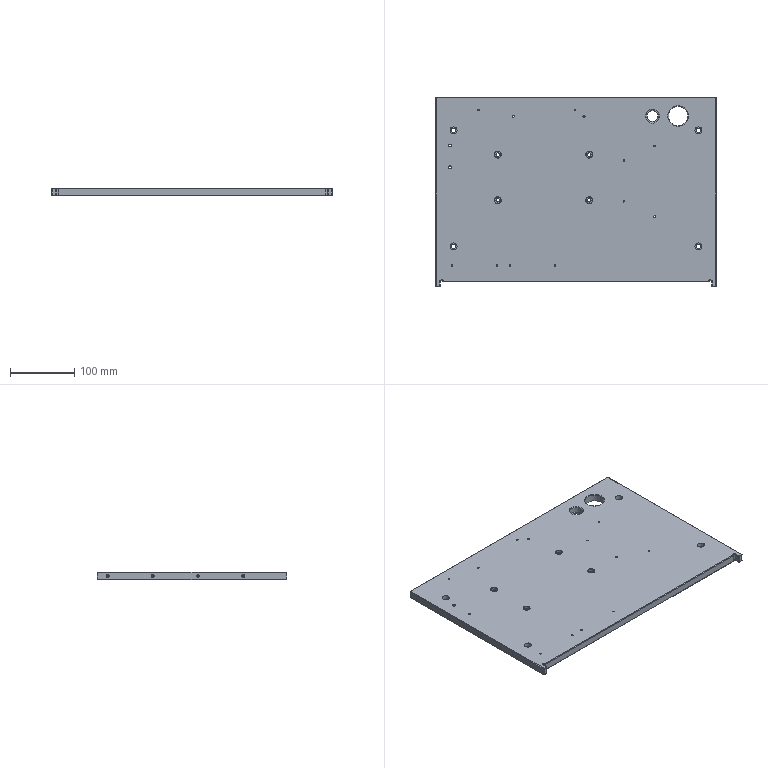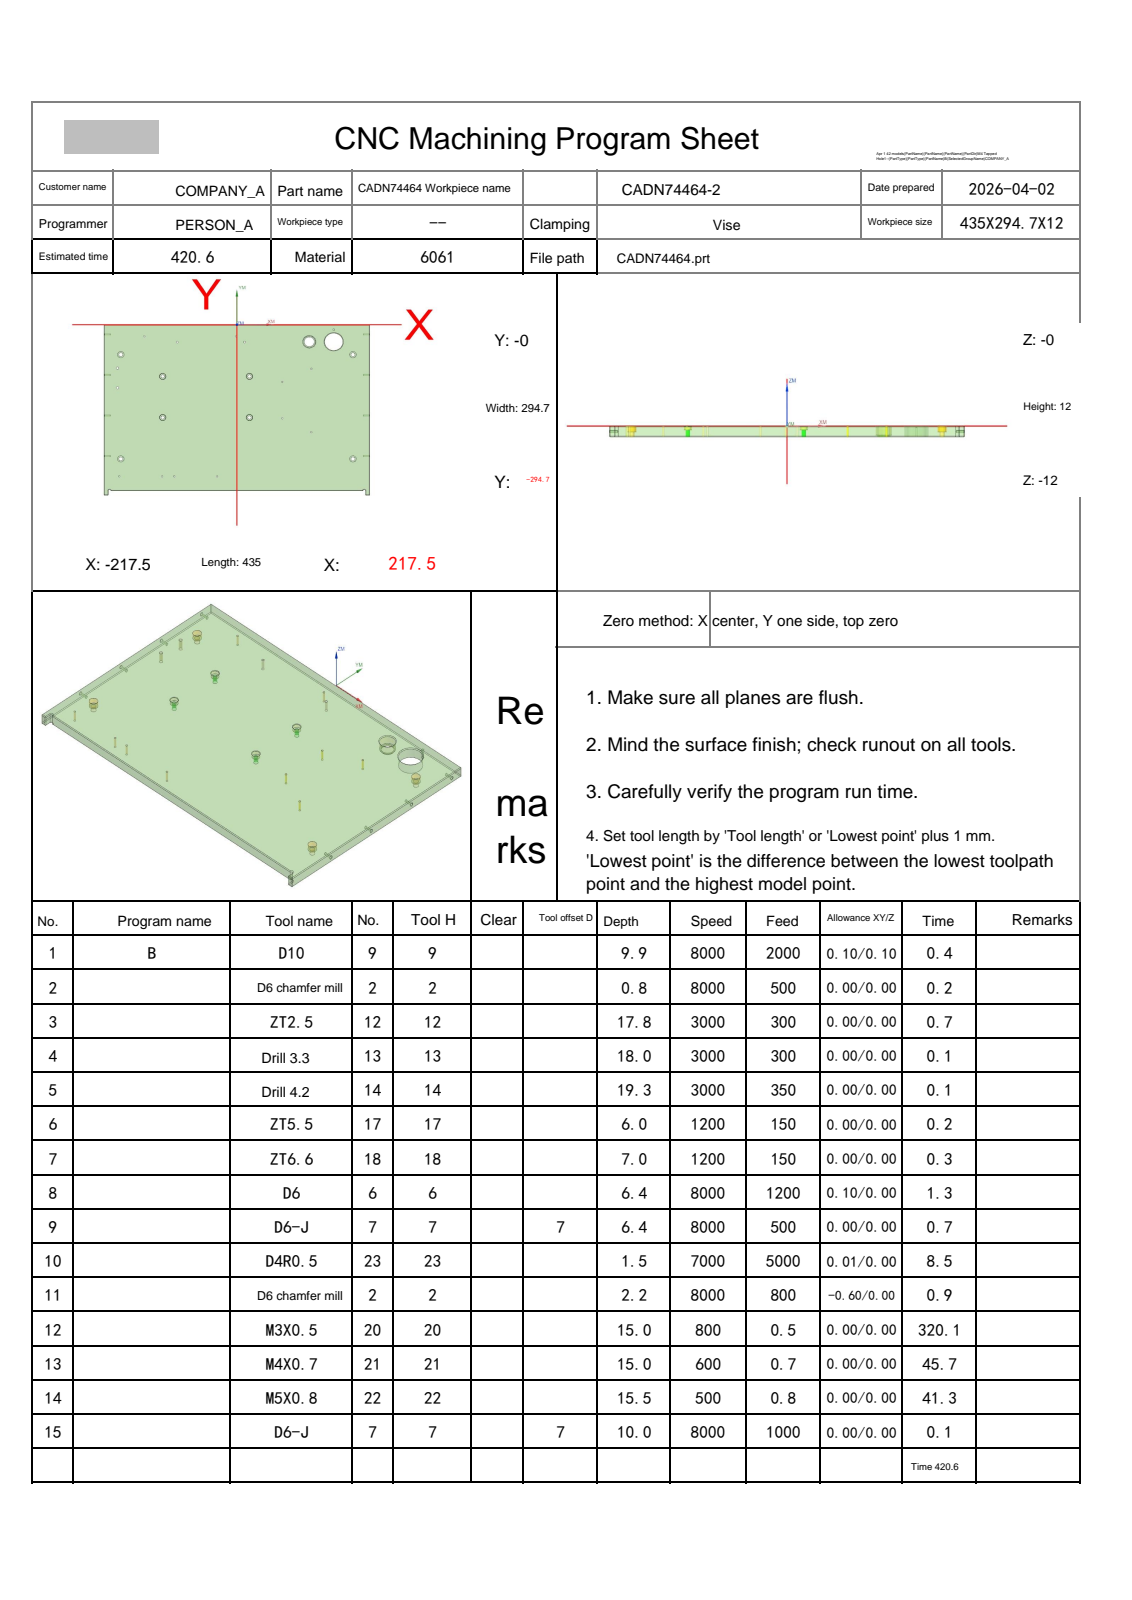NC program | NX | posted by the shop | part box 435 x 294.7 x 12 mm
Lines 634 to 1915 of 33933:
N10 T23 M06
(D4R0.5  D=4. R=0.5 H=23 ce=0.01 di=0.00)
G00 G90 G54 X119.057 Y-38.818 M03 S7000
G43 H23 Z20.
M08
Z1.5
G01 X119.198 Y-38.814 Z1.493 F5000.
X120.02 Y-38.715 Z1.449
X120.831 Y-38.544 Z1.406
X121.624 Y-38.302 Z1.362
X122.392 Y-37.991 Z1.319
X123.129 Y-37.612 Z1.276
X123.83 Y-37.17 Z1.232
X124.488 Y-36.668 Z1.189
X125.1 Y-36.109 Z1.145
X125.66 Y-35.498 Z1.102
X126.163 Y-34.839 Z1.058
X126.496 Y-34.327 Z1.026
X126.905 Y-33.574 Z.981
X127.243 Y-32.786 Z.937
X127.507 Y-31.971 Z.892
X127.696 Y-31.136 Z.847
X127.807 Y-30.286 Z.802
X127.84 Y-29.43 Z.757
X127.794 Y-28.574 Z.712
X127.67 Y-27.727 Z.667
X127.469 Y-26.894 Z.622
X127.192 Y-26.083 Z.577
X126.843 Y-25.301 Z.532
X126.423 Y-24.554 Z.488
X125.936 Y-23.849 Z.443
X125.387 Y-23.191 Z.398
X124.78 Y-22.586 Z.353
X124.12 Y-22.04 Z.308
X123.413 Y-21.556 Z.263
X122.664 Y-21.14 Z.218
X121.881 Y-20.793 Z.173
X121.068 Y-20.52 Z.128
X120.476 Y-20.371 Z.096
X119.645 Y-20.23 Z.052
X118.806 Y-20.165 Z.008
X118.5 Z-.008
G03 X109.165 Y-29.5 I0.0 J-9.335
X118.5 Y-38.835 I9.335 J0.0
X127.835 Y-29.5 I0.0 J9.335
X118.5 Y-20.165 I-9.335 J0.0
G01 X118.269 Y-20.168
X118.038 Y-20.177
X117.802 Y-20.192
X117.567 Y-20.213
X117.27 Y-20.248
X116.974 Y-20.293
X116.675 Y-20.348
X116.378 Y-20.413
X116.083 Y-20.488 Z-.009
X115.791 Y-20.572
X115.502 Y-20.665
X115.216 Y-20.768
X114.934 Y-20.88
X114.655 Y-21.002
X114.518 Y-21.066
X114.381 Y-21.132
X114.245 Y-21.2
X114.111 Y-21.271
X113.978 Y-21.344
X113.846 Y-21.419
X113.715 Y-21.496
X113.585 Y-21.575
X113.457 Y-21.657
X113.33 Y-21.74
X113.205 Y-21.826
X113.081 Y-21.913
X112.958 Y-22.003
X112.836 Y-22.094
X112.717 Y-22.187
X112.599 Y-22.283
X112.482 Y-22.38
X112.367 Y-22.479
X112.254 Y-22.58 Z-.01
X112.142 Y-22.683
X112.032 Y-22.788
X111.924 Y-22.894
X111.817 Y-23.002
X111.713 Y-23.113
X111.61 Y-23.224
X111.509 Y-23.337
X111.41 Y-23.452
X111.312 Y-23.569
X111.217 Y-23.687
X111.123 Y-23.806
X111.032 Y-23.927
X110.942 Y-24.05
X110.855 Y-24.174
X110.769 Y-24.299
X110.686 Y-24.426
X110.604 Y-24.554
X110.448 Y-24.814
X110.3 Y-25.079
X110.161 Y-25.348
X110.031 Y-25.622
X109.909 Y-25.901
X109.797 Y-26.182
X109.694 Y-26.468 Z-.011
X109.601 Y-26.756
X109.517 Y-27.048
X109.442 Y-27.342
X109.377 Y-27.638
X109.322 Y-27.936
X109.276 Y-28.236
X109.24 Y-28.537
X109.215 Y-28.839
X109.198 Y-29.142
X109.192 Y-29.445
X109.196 Y-29.748
X109.21 Y-30.051
X109.233 Y-30.353
X109.266 Y-30.655
X109.309 Y-30.955 Z-.012
X109.362 Y-31.253
X109.424 Y-31.55
X109.497 Y-31.844
X109.578 Y-32.136
X109.669 Y-32.425
X109.769 Y-32.711
X109.879 Y-32.993
X109.998 Y-33.272
X110.126 Y-33.546
X110.263 Y-33.817
X110.408 Y-34.082
X110.562 Y-34.343
X110.577 Y-34.367
X110.592 Y-34.392
X110.74 Y-34.623
X110.895 Y-34.849
X111.073 Y-35.093
X111.26 Y-35.332 Z-.013
X111.454 Y-35.564
X111.655 Y-35.79
X111.864 Y-36.009
X112.079 Y-36.221
X112.302 Y-36.426
X112.531 Y-36.623
X112.648 Y-36.719
X112.766 Y-36.813
X112.886 Y-36.906
X113.007 Y-36.996
X113.13 Y-37.084
X113.254 Y-37.17
X113.38 Y-37.254
X113.507 Y-37.336
X113.635 Y-37.416
X113.765 Y-37.494
X113.896 Y-37.57
X114.028 Y-37.643
X114.161 Y-37.715
X114.295 Y-37.785
X114.431 Y-37.852
X114.568 Y-37.916
X114.705 Y-37.979
X114.844 Y-38.04 Z-.014
X114.983 Y-38.098
X115.124 Y-38.153
X115.265 Y-38.207
X115.407 Y-38.258
X115.55 Y-38.307
X115.694 Y-38.354
X115.839 Y-38.398
X115.984 Y-38.44
X116.13 Y-38.48
X116.276 Y-38.517
X116.423 Y-38.551
X116.571 Y-38.584
X116.719 Y-38.614
X116.868 Y-38.641
X117.017 Y-38.666
X117.166 Y-38.689
X117.316 Y-38.709
X117.466 Y-38.727
X117.616 Y-38.743
X117.767 Y-38.756
X117.917 Y-38.766
X118.068 Y-38.774
X118.37 Y-38.783
X118.672 Y-38.782
X118.974 Y-38.771
X119.276 Y-38.75 Z-.015
X119.576 Y-38.719
X119.876 Y-38.679
X120.173 Y-38.629
X120.47 Y-38.569
X120.763 Y-38.5
X121.055 Y-38.421
X121.344 Y-38.333
X121.63 Y-38.235
X121.912 Y-38.128
X122.191 Y-38.012
X122.466 Y-37.887
X122.736 Y-37.753
X123.002 Y-37.61
X123.264 Y-37.459
X123.52 Y-37.3
X123.771 Y-37.132 Z-.016
X124.016 Y-36.956
X124.256 Y-36.772
X124.489 Y-36.581
X124.716 Y-36.382
X124.936 Y-36.175
X125.15 Y-35.962
X125.356 Y-35.742
X125.555 Y-35.515
X125.747 Y-35.282
X125.931 Y-35.043
X126.089 Y-34.823
X126.242 Y-34.598
X126.258 Y-34.573
X126.275 Y-34.548
X126.43 Y-34.298
X126.578 Y-34.045
X126.718 Y-33.786 Z-.017
X126.849 Y-33.524
X126.972 Y-33.257
X127.086 Y-32.987
X127.192 Y-32.713
X127.289 Y-32.436
X127.377 Y-32.156
X127.457 Y-31.873
X127.527 Y-31.588
X127.588 Y-31.301
X127.64 Y-31.012
X127.683 Y-30.722
X127.716 Y-30.431
X127.741 Y-30.138
X127.756 Y-29.845
X127.762 Y-29.552
X127.759 Y-29.258 Z-.018
X127.746 Y-28.965
X127.724 Y-28.673
X127.693 Y-28.381
X127.652 Y-28.091
X127.602 Y-27.801
X127.544 Y-27.514
X127.476 Y-27.229
X127.399 Y-26.946
X127.313 Y-26.665
X127.219 Y-26.388
X127.115 Y-26.113
X127.003 Y-25.842
X126.883 Y-25.575
X126.754 Y-25.311
X126.617 Y-25.052
X126.472 Y-24.798 Z-.019
X126.318 Y-24.548
X126.157 Y-24.303
X125.988 Y-24.063
X125.812 Y-23.829
X125.628 Y-23.6
X125.438 Y-23.378
X125.24 Y-23.161
X125.036 Y-22.951
X124.825 Y-22.748
X124.607 Y-22.551
X124.384 Y-22.362
X124.155 Y-22.179
X123.92 Y-22.004
X123.679 Y-21.836
X123.434 Y-21.677
X123.183 Y-21.525 Z-.02
X122.928 Y-21.381
X122.669 Y-21.245
X122.405 Y-21.117
X122.137 Y-20.998
X121.866 Y-20.887
X121.591 Y-20.786
X121.314 Y-20.692
X121.033 Y-20.608
X120.75 Y-20.532
X120.553 Y-20.486
X120.355 Y-20.443
X120.275 Y-20.428
X120.195 Y-20.412
X119.915 Y-20.365
X119.634 Y-20.326
X119.351 Y-20.296
X119.068 Y-20.274
X118.784 Y-20.262 Z-.021
X118.5 Y-20.258
X118.269 Y-20.261
X118.038 Y-20.27
X117.802 Y-20.285
X117.567 Y-20.306
X117.272 Y-20.342
X116.978 Y-20.386
X116.682 Y-20.441
X116.387 Y-20.506
X116.095 Y-20.58
X115.805 Y-20.664
X115.518 Y-20.757 Z-.022
X115.234 Y-20.86
X114.954 Y-20.972
X114.678 Y-21.093
X114.541 Y-21.156
X114.406 Y-21.222
X114.271 Y-21.291
X114.138 Y-21.361
X114.006 Y-21.433
X113.875 Y-21.508
X113.745 Y-21.585
X113.617 Y-21.664
X113.489 Y-21.745
X113.364 Y-21.828
X113.239 Y-21.913
X113.116 Y-22.
X112.995 Y-22.089
X112.874 Y-22.18
X112.756 Y-22.273 Z-.023
X112.639 Y-22.368
X112.523 Y-22.465
X112.409 Y-22.564
X112.297 Y-22.664
X112.187 Y-22.767
X112.078 Y-22.871
X111.97 Y-22.977
X111.865 Y-23.085
X111.761 Y-23.194
X111.659 Y-23.305
X111.559 Y-23.418
X111.461 Y-23.532
X111.365 Y-23.648
X111.271 Y-23.765
X111.178 Y-23.884
X111.088 Y-24.005
X110.999 Y-24.127
X110.828 Y-24.375
X110.665 Y-24.628
X110.511 Y-24.887 Z-.024
X110.365 Y-25.15
X110.228 Y-25.418
X110.099 Y-25.691
X109.98 Y-25.967
X109.869 Y-26.248
X109.768 Y-26.531
X109.676 Y-26.818
X109.594 Y-27.108
X109.521 Y-27.4
X109.458 Y-27.694
X109.404 Y-27.991 Z-.025
X109.36 Y-28.288
X109.326 Y-28.588
X109.302 Y-28.888
X109.287 Y-29.188
X109.283 Y-29.489
X109.287 Y-29.79
X109.302 Y-30.091
X109.327 Y-30.391
X109.362 Y-30.69
X109.406 Y-30.987
X109.46 Y-31.283 Z-.026
X109.523 Y-31.578
X109.596 Y-31.869
X109.679 Y-32.159
X109.771 Y-32.445
X109.872 Y-32.728
X109.983 Y-33.008
X110.102 Y-33.284
X110.231 Y-33.556
X110.368 Y-33.824
X110.514 Y-34.087
X110.668 Y-34.345 Z-.027
X110.683 Y-34.368
X110.697 Y-34.392
X110.845 Y-34.618
X110.998 Y-34.84
X111.175 Y-35.08
X111.36 Y-35.314
X111.552 Y-35.541
X111.751 Y-35.762
X111.958 Y-35.977
X112.171 Y-36.185
X112.391 Y-36.385
X112.617 Y-36.579
X112.849 Y-36.765 Z-.028
X113.087 Y-36.944
X113.331 Y-37.115
X113.58 Y-37.277
X113.835 Y-37.432
X114.094 Y-37.578
X114.358 Y-37.716
X114.626 Y-37.845
X114.898 Y-37.966
X115.174 Y-38.077
X115.313 Y-38.13
X115.453 Y-38.18
X115.594 Y-38.228 Z-.029
X115.735 Y-38.273
X115.878 Y-38.317
X116.021 Y-38.358
X116.164 Y-38.397
X116.308 Y-38.433
X116.453 Y-38.467
X116.599 Y-38.499
X116.744 Y-38.528
X116.891 Y-38.555
X117.037 Y-38.58
X117.184 Y-38.602
X117.332 Y-38.622
X117.479 Y-38.639
X117.776 Y-38.667
X118.072 Y-38.685
X118.37 Y-38.694
X118.667 Y-38.693
X118.964 Y-38.682 Z-.03
X119.261 Y-38.662
X119.557 Y-38.632
X119.851 Y-38.593
X120.145 Y-38.544
X120.436 Y-38.486
X120.726 Y-38.418
X121.013 Y-38.341
X121.297 Y-38.254
X121.579 Y-38.159
X121.857 Y-38.055
X122.132 Y-37.941 Z-.031
X122.402 Y-37.819
X122.669 Y-37.688
X122.931 Y-37.548
X123.189 Y-37.401
X123.442 Y-37.244
X123.69 Y-37.08
X123.932 Y-36.908
X124.168 Y-36.728
X124.399 Y-36.541
X124.623 Y-36.346
X124.841 Y-36.144 Z-.032
X125.052 Y-35.935
X125.256 Y-35.72
X125.454 Y-35.498
X125.644 Y-35.269
X125.826 Y-35.035
X126.001 Y-34.795
X126.168 Y-34.55
X126.224 Y-34.463
X126.279 Y-34.377
X126.381 Y-34.209
X126.479 Y-34.04
X126.622 Y-33.778
X126.757 Y-33.512 Z-.033
X126.882 Y-33.241
X126.999 Y-32.966
X127.107 Y-32.688
X127.206 Y-32.406
X127.295 Y-32.121
X127.375 Y-31.834
X127.446 Y-31.544
X127.507 Y-31.252
X127.559 Y-30.958
X127.601 Y-30.663
X127.634 Y-30.366 Z-.034
X127.657 Y-30.069
X127.67 Y-29.771
X127.674 Y-29.472
X127.667 Y-29.174
X127.652 Y-28.876
X127.626 Y-28.579
X127.591 Y-28.283
X127.546 Y-27.988
X127.492 Y-27.695
X127.428 Y-27.404
X127.355 Y-27.115 Z-.035
X127.272 Y-26.828
X127.18 Y-26.544
X127.079 Y-26.264
X126.969 Y-25.987
X126.85 Y-25.713
X126.722 Y-25.444
X126.585 Y-25.179
X126.44 Y-24.919
X126.364 Y-24.79
X126.287 Y-24.663
X126.207 Y-24.537
X126.125 Y-24.413
X126.041 Y-24.29
X125.955 Y-24.168 Z-.036
X125.867 Y-24.048
X125.777 Y-23.929
X125.686 Y-23.811
X125.592 Y-23.695
X125.497 Y-23.581
X125.399 Y-23.468
X125.3 Y-23.357
X125.199 Y-23.247
X125.097 Y-23.139
X124.992 Y-23.033
X124.886 Y-22.928
X124.778 Y-22.825
X124.669 Y-22.724
X124.558 Y-22.625
X124.331 Y-22.432
X124.097 Y-22.247
X123.859 Y-22.069
X123.614 Y-21.899 Z-.037
X123.364 Y-21.737
X123.109 Y-21.583
X122.849 Y-21.438
X122.584 Y-21.301
X122.315 Y-21.173
X122.042 Y-21.054
X121.766 Y-20.943
X121.485 Y-20.842
X121.202 Y-20.75
X120.916 Y-20.667
X120.628 Y-20.594 Z-.038
X120.337 Y-20.53
X120.11 Y-20.487
X119.882 Y-20.449
X119.864 Y-20.447
X119.847 Y-20.444
X119.635 Y-20.415
X119.423 Y-20.391
X119.193 Y-20.371
X118.962 Y-20.357
X118.731 Y-20.349
X118.5 Y-20.346
X118.269 Y-20.349
X118.038 Y-20.358
X117.807 Y-20.374
X117.576 Y-20.394 Z-.039
X117.461 Y-20.407
X117.345 Y-20.421
X117.164 Y-20.446
X116.983 Y-20.475
X116.688 Y-20.53
X116.396 Y-20.595
X116.106 Y-20.669
X115.818 Y-20.752
X115.533 Y-20.845
X115.252 Y-20.948
X114.974 Y-21.059 Z-.04
X114.7 Y-21.179
X114.564 Y-21.243
X114.43 Y-21.309
X114.296 Y-21.377
X114.164 Y-21.447
X114.033 Y-21.519
X113.903 Y-21.593
X113.774 Y-21.67
X113.647 Y-21.749
X113.521 Y-21.829
X113.396 Y-21.912
X113.273 Y-21.997
X113.151 Y-22.084
X113.03 Y-22.172
X112.911 Y-22.263 Z-.041
X112.793 Y-22.356
X112.678 Y-22.45
X112.563 Y-22.547
X112.45 Y-22.645
X112.339 Y-22.745
X112.229 Y-22.847
X112.121 Y-22.951
X112.015 Y-23.056
X111.911 Y-23.163
X111.808 Y-23.272
X111.707 Y-23.383
X111.608 Y-23.495
X111.511 Y-23.609
X111.416 Y-23.724
X111.231 Y-23.959
X111.054 Y-24.2 Z-.042
X110.885 Y-24.447
X110.724 Y-24.699
X110.571 Y-24.957
X110.427 Y-25.219
X110.292 Y-25.486
X110.165 Y-25.757
X110.048 Y-26.032
X109.939 Y-26.31
X109.84 Y-26.592 Z-.043
X109.75 Y-26.877
X109.669 Y-27.165
X109.598 Y-27.456
X109.536 Y-27.748
X109.484 Y-28.043
X109.442 Y-28.339
X109.409 Y-28.636
X109.386 Y-28.934 Z-.044
X109.373 Y-29.233
X109.37 Y-29.531
X109.376 Y-29.83
X109.392 Y-30.129
X109.418 Y-30.426
X109.454 Y-30.723
X109.499 Y-31.019
X109.554 Y-31.312
X109.618 Y-31.604 Z-.045
X109.693 Y-31.893
X109.776 Y-32.18
X109.869 Y-32.464
X109.971 Y-32.745
X110.082 Y-33.022
X110.202 Y-33.296
X110.332 Y-33.565
X110.469 Y-33.83 Z-.046
X110.616 Y-34.09
X110.771 Y-34.346
X110.785 Y-34.368
X110.799 Y-34.391
X110.948 Y-34.617
X111.104 Y-34.838
X111.282 Y-35.076
X111.468 Y-35.309
X111.661 Y-35.534
X111.862 Y-35.754
X112.07 Y-35.967 Z-.047
X112.284 Y-36.172
X112.506 Y-36.371
X112.733 Y-36.563
X112.967 Y-36.746
X113.206 Y-36.923
X113.451 Y-37.091
X113.702 Y-37.251
X113.957 Y-37.403
X114.217 Y-37.546 Z-.048
X114.482 Y-37.681
X114.751 Y-37.808
X115.024 Y-37.925
X115.301 Y-38.033
X115.581 Y-38.133
X115.864 Y-38.223
X116.007 Y-38.265
X116.15 Y-38.304
X116.294 Y-38.341
X116.438 Y-38.375 Z-.049
X116.583 Y-38.408
X116.729 Y-38.437
X116.875 Y-38.465
X117.021 Y-38.49
X117.168 Y-38.513
X117.315 Y-38.533
X117.463 Y-38.551
X117.61 Y-38.566
X117.906 Y-38.59
X118.203 Y-38.604
X118.5 Y-38.609
X118.797 Y-38.603
X119.094 Y-38.588 Z-.05
X119.389 Y-38.564
X119.684 Y-38.53
X119.978 Y-38.486
X120.27 Y-38.432
X120.56 Y-38.369
X120.848 Y-38.297
X121.134 Y-38.215
X121.416 Y-38.125 Z-.051
X121.696 Y-38.024
X121.972 Y-37.915
X122.244 Y-37.797
X122.512 Y-37.67
X122.777 Y-37.535
X123.036 Y-37.391
X123.291 Y-37.238
X123.54 Y-37.078
X123.784 Y-36.909 Z-.052
X124.023 Y-36.732
X124.255 Y-36.548
X124.482 Y-36.357
X124.702 Y-36.158
X124.915 Y-35.952
X125.122 Y-35.739
X125.321 Y-35.519
X125.514 Y-35.293
X125.698 Y-35.061 Z-.053
X125.876 Y-34.824
X126.047 Y-34.577
X126.21 Y-34.324
X126.363 Y-34.07
X126.508 Y-33.811
X126.645 Y-33.544
X126.774 Y-33.272
X126.894 Y-32.997 Z-.054
X127.005 Y-32.717
X127.106 Y-32.434
X127.198 Y-32.148
X127.28 Y-31.859
X127.353 Y-31.568
X127.416 Y-31.274
X127.469 Y-30.978
X127.513 Y-30.681
X127.546 Y-30.382 Z-.055
X127.57 Y-30.083
X127.584 Y-29.783
X127.588 Y-29.482
X127.582 Y-29.182
X127.566 Y-28.882
X127.54 Y-28.583
X127.505 Y-28.285
X127.459 Y-27.988 Z-.056
X127.404 Y-27.693
X127.339 Y-27.4
X127.264 Y-27.109
X127.18 Y-26.821
X127.086 Y-26.535
X126.983 Y-26.253
X126.928 Y-26.114
X126.871 Y-25.975
X126.811 Y-25.837
X126.75 Y-25.7
X126.685 Y-25.565 Z-.057
X126.619 Y-25.43
X126.551 Y-25.297
X126.48 Y-25.164
X126.407 Y-25.033
X126.332 Y-24.903
X126.255 Y-24.774
X126.175 Y-24.647
X126.094 Y-24.521
X126.01 Y-24.396
X125.925 Y-24.273
X125.837 Y-24.151
X125.748 Y-24.031
X125.656 Y-23.912
X125.563 Y-23.794
X125.467 Y-23.679
X125.37 Y-23.564
X125.271 Y-23.452 Z-.058
X125.17 Y-23.341
X125.067 Y-23.232
X124.962 Y-23.124
X124.856 Y-23.018
X124.748 Y-22.914
X124.638 Y-22.812
X124.526 Y-22.712
X124.413 Y-22.613
X124.299 Y-22.517
X124.182 Y-22.422
X124.064 Y-22.329
X123.945 Y-22.238
X123.824 Y-22.15
X123.702 Y-22.063
X123.578 Y-21.978
X123.453 Y-21.895
X123.327 Y-21.815 Z-.059
X123.199 Y-21.736
X123.07 Y-21.66
X122.939 Y-21.585
X122.808 Y-21.513
X122.675 Y-21.443
X122.541 Y-21.376
X122.407 Y-21.31
X122.271 Y-21.247
X122.134 Y-21.186
X121.857 Y-21.071
X121.576 Y-20.965
X121.292 Y-20.868
X121.005 Y-20.781
X120.779 Y-20.719 Z-.06
X120.552 Y-20.664
X120.488 Y-20.649
X120.424 Y-20.635
X120.13 Y-20.577
X119.834 Y-20.528
X119.613 Y-20.499
X119.391 Y-20.474
X119.169 Y-20.455
X118.946 Y-20.442
X118.723 Y-20.434
X118.5 Y-20.432
X118.213 Y-20.436 Z-.061
X117.927 Y-20.45
X117.747 Y-20.464
X117.568 Y-20.481
X117.462 Y-20.493
X117.356 Y-20.506
X117.065 Y-20.548
X116.775 Y-20.6
X116.488 Y-20.661
X116.203 Y-20.731 Z-.062
X115.92 Y-20.811
X115.64 Y-20.899
X115.362 Y-20.997
X115.089 Y-21.104
X114.818 Y-21.219
X114.552 Y-21.343
X114.29 Y-21.476 Z-.063
X114.032 Y-21.617
X113.779 Y-21.766
X113.532 Y-21.924
X113.289 Y-22.089
X113.052 Y-22.263
X112.82 Y-22.443
X112.595 Y-22.632 Z-.064
X112.375 Y-22.827
X112.163 Y-23.029
X111.957 Y-23.238
X111.757 Y-23.454
X111.565 Y-23.676
X111.381 Y-23.904
X111.203 Y-24.138 Z-.065
X111.034 Y-24.378
X110.872 Y-24.623
X110.718 Y-24.873
X110.573 Y-25.128
X110.436 Y-25.387
X110.307 Y-25.651
X110.187 Y-25.919 Z-.066
X110.076 Y-26.19
X109.973 Y-26.465
X109.88 Y-26.743
X109.795 Y-27.024
X109.72 Y-27.308
X109.654 Y-27.594
X109.597 Y-27.882 Z-.067
X109.55 Y-28.171
X109.512 Y-28.462
X109.484 Y-28.754
X109.465 Y-29.047
X109.455 Y-29.34
Y-29.633
X109.465 Y-29.926
X109.484 Y-30.219 Z-.068
X109.512 Y-30.511
X109.55 Y-30.801
X109.597 Y-31.091
X109.654 Y-31.378
X109.72 Y-31.664
X109.795 Y-31.947
X109.88 Y-32.228 Z-.069
X109.973 Y-32.506
X110.075 Y-32.781
X110.187 Y-33.052
X110.306 Y-33.319
X110.435 Y-33.583
X110.572 Y-33.842
X110.665 Y-34.006 Z-.07
X110.761 Y-34.169
X110.815 Y-34.258
X110.871 Y-34.346
X111.033 Y-34.591
X111.203 Y-34.831
X111.38 Y-35.065
X111.565 Y-35.294
X111.758 Y-35.516
X111.957 Y-35.732 Z-.071
X112.164 Y-35.941
X112.377 Y-36.143
X112.596 Y-36.338
X112.822 Y-36.526
X113.054 Y-36.707
X113.291 Y-36.88
X113.534 Y-37.045 Z-.072
X113.783 Y-37.202
X114.036 Y-37.351
X114.294 Y-37.492
X114.556 Y-37.624
X114.822 Y-37.747
X115.093 Y-37.862
X115.367 Y-37.968 Z-.073
X115.644 Y-38.065
X115.924 Y-38.153
X116.207 Y-38.232
X116.492 Y-38.301
X116.779 Y-38.362
X117.069 Y-38.412
X117.359 Y-38.454 Z-.074
X117.651 Y-38.486
X117.944 Y-38.508
X118.237 Y-38.521
X118.531 Y-38.525
X118.824 Y-38.518
X119.117 Y-38.503
X119.41 Y-38.477 Z-.075
X119.701 Y-38.443
X119.991 Y-38.398
X120.28 Y-38.345
X120.566 Y-38.282
X120.851 Y-38.21
X121.132 Y-38.128
X121.411 Y-38.038
X121.687 Y-37.938 Z-.076
X121.96 Y-37.829
X122.229 Y-37.712
X122.494 Y-37.586
X122.754 Y-37.452
X123.01 Y-37.309
X123.262 Y-37.158
X123.508 Y-36.998 Z-.077
X123.749 Y-36.831
X123.984 Y-36.656
X124.214 Y-36.474
X124.437 Y-36.284
X124.655 Y-36.087
X124.865 Y-35.883
X125.069 Y-35.672 Z-.078
X125.266 Y-35.455
X125.456 Y-35.232
X125.638 Y-35.002
X125.813 Y-34.767
X125.948 Y-34.573
X126.078 Y-34.377
X126.109 Y-34.328
X126.139 Y-34.28
X126.292 Y-34.027 Z-.079
X126.436 Y-33.769
X126.571 Y-33.506
X126.697 Y-33.239
X126.815 Y-32.968
X126.924 Y-32.694
X127.024 Y-32.416
X127.114 Y-32.135 Z-.08
X127.196 Y-31.851
X127.268 Y-31.564
X127.33 Y-31.276
X127.383 Y-30.985
X127.427 Y-30.693
X127.461 Y-30.4
X127.485 Y-30.105 Z-.081
X127.5 Y-29.81
X127.504 Y-29.515
X127.5 Y-29.22
X127.485 Y-28.925
X127.461 Y-28.631
X127.427 Y-28.338
X127.384 Y-28.046 Z-.082
X127.331 Y-27.755
X127.269 Y-27.467
X127.197 Y-27.181
X127.116 Y-26.897
X127.026 Y-26.616
X126.926 Y-26.338
X126.818 Y-26.064 Z-.083
X126.7 Y-25.793
X126.574 Y-25.526
X126.439 Y-25.264
X126.295 Y-25.006
X126.143 Y-24.753
X125.983 Y-24.506
X125.815 Y-24.263 Z-.084
X125.639 Y-24.026
X125.456 Y-23.796
X125.265 Y-23.571
X125.066 Y-23.353
X124.861 Y-23.141
X124.649 Y-22.936
X124.54 Y-22.836
X124.43 Y-22.738
X124.318 Y-22.642 Z-.085
X124.205 Y-22.548
X123.974 Y-22.365
X123.737 Y-22.19
X123.494 Y-22.022
X123.246 Y-21.863
X122.993 Y-21.712
X122.735 Y-21.569
X122.473 Y-21.435 Z-.086
X122.206 Y-21.309
X121.935 Y-21.192
X121.661 Y-21.085
X121.383 Y-20.986
X121.102 Y-20.896
X120.819 Y-20.816
X120.533 Y-20.745 Z-.087
X120.339 Y-20.703
X120.144 Y-20.664
X120.087 Y-20.654
X120.03 Y-20.644
X119.777 Y-20.604
X119.523 Y-20.572
X119.268 Y-20.547
X119.012 Y-20.529
X118.756 Y-20.518
X118.5 Y-20.515 Z-.088
X118.269 Y-20.518
X118.038 Y-20.527
X117.803 Y-20.543
X117.568 Y-20.565
X117.283 Y-20.6
X116.999 Y-20.644
X116.713 Y-20.697 Z-.089
X116.429 Y-20.76
X116.147 Y-20.832
X115.867 Y-20.914
X115.59 Y-21.004
X115.316 Y-21.103
X115.046 Y-21.211 Z-.09
X114.779 Y-21.328
X114.516 Y-21.454
X114.258 Y-21.587
X114.004 Y-21.729
X113.754 Y-21.88
X113.51 Y-22.038 Z-.091
X113.271 Y-22.204
X113.037 Y-22.378
X112.81 Y-22.559
X112.588 Y-22.748
X112.372 Y-22.943
X112.163 Y-23.146 Z-.092
X111.961 Y-23.355
X111.765 Y-23.57
X111.577 Y-23.792
X111.396 Y-24.02
X111.222 Y-24.253
X111.056 Y-24.492 Z-.093
X110.898 Y-24.736
X110.748 Y-24.986
X110.606 Y-25.24
X110.473 Y-25.498
X110.348 Y-25.76
X110.231 Y-26.027 Z-.094
X110.123 Y-26.297
X110.024 Y-26.571
X109.934 Y-26.847
X109.853 Y-27.126
X109.781 Y-27.408
X109.718 Y-27.692 Z-.095
X109.664 Y-27.978
X109.62 Y-28.265
X109.585 Y-28.554
X109.56 Y-28.843
X109.543 Y-29.133
X109.537 Y-29.424 Z-.096
X109.539 Y-29.715
X109.552 Y-30.005
X109.573 Y-30.295
X109.604 Y-30.584
X109.644 Y-30.872
X109.694 Y-31.158 Z-.097
X109.753 Y-31.443
X109.821 Y-31.725
X109.898 Y-32.005
X109.984 Y-32.283
X110.079 Y-32.557
X110.183 Y-32.828
X110.296 Y-33.096 Z-.098
X110.417 Y-33.36
X110.547 Y-33.62
X110.685 Y-33.875
X110.831 Y-34.126
X110.844 Y-34.147
X110.857 Y-34.169
X111.001 Y-34.395
X111.151 Y-34.617 Z-.099
X111.322 Y-34.854
X111.501 Y-35.086
X111.688 Y-35.311
X111.882 Y-35.531
X112.083 Y-35.743
X112.291 Y-35.949 Z-.1
X112.505 Y-36.149
X112.726 Y-36.341
X112.953 Y-36.525
X113.186 Y-36.703
X113.424 Y-36.872
X113.668 Y-37.034 Z-.101
X113.917 Y-37.187
X114.171 Y-37.333
X114.43 Y-37.47
X114.693 Y-37.598
X114.96 Y-37.718
X115.23 Y-37.829 Z-.102
X115.504 Y-37.931
X115.782 Y-38.024
X116.062 Y-38.108
X116.345 Y-38.182
X116.63 Y-38.248
X116.917 Y-38.304 Z-.103
X117.205 Y-38.35
X117.495 Y-38.387
X117.786 Y-38.415
X118.078 Y-38.433
X118.37 Y-38.442
X118.663 Y-38.441 Z-.104
X118.955 Y-38.43
X119.247 Y-38.41
X119.537 Y-38.381
X119.827 Y-38.342
X120.115 Y-38.293
X120.402 Y-38.235 Z-.105
X120.686 Y-38.168
X120.968 Y-38.091
X121.248 Y-38.006
X121.524 Y-37.911
X121.797 Y-37.807
X122.067 Y-37.695 Z-.106
X122.333 Y-37.573
X122.594 Y-37.443
X122.851 Y-37.305
X123.104 Y-37.158
X123.352 Y-37.003
X123.594 Y-36.84 Z-.107
X123.831 Y-36.67
X124.062 Y-36.491
X124.288 Y-36.305
X124.507 Y-36.112
X124.719 Y-35.912
X124.925 Y-35.705 Z-.108
X125.124 Y-35.491
X125.316 Y-35.271
X125.501 Y-35.045
X125.678 Y-34.813
X125.837 Y-34.591
X125.989 Y-34.364 Z-.109
X125.999 Y-34.348
X126.01 Y-34.332
X126.163 Y-34.084
X126.308 Y-33.832
X126.445 Y-33.574
X126.573 Y-33.313
X126.693 Y-33.047
X126.804 Y-32.778 Z-.11
X126.906 Y-32.505
X126.999 Y-32.229
X127.084 Y-31.95
X127.159 Y-31.668
X127.224 Y-31.384
X127.281 Y-31.098 Z-.111
X127.328 Y-30.811
X127.366 Y-30.522
X127.394 Y-30.232
X127.413 Y-29.941
X127.422 Y-29.65
Y-29.359 Z-.112
X127.412 Y-29.068
X127.393 Y-28.777
X127.364 Y-28.488
X127.326 Y-28.199
X127.278 Y-27.912
X127.221 Y-27.626 Z-.113
X127.155 Y-27.342
X127.08 Y-27.061
X126.995 Y-26.783
X126.901 Y-26.507
X126.799 Y-26.234
X126.687 Y-25.966 Z-.114
X126.567 Y-25.7
X126.439 Y-25.439
X126.302 Y-25.183
X126.156 Y-24.93
X126.003 Y-24.683
X125.841 Y-24.441
X125.672 Y-24.204 Z-.115
X125.495 Y-23.973
X125.31 Y-23.748
X125.119 Y-23.529
X124.92 Y-23.317
X124.714 Y-23.111
X124.502 Y-22.912 Z-.116
X124.284 Y-22.72
X124.059 Y-22.535
X123.829 Y-22.357
X123.593 Y-22.188
X123.351 Y-22.026
X123.104 Y-21.872 Z-.117
X122.853 Y-21.726
X122.596 Y-21.588
X122.336 Y-21.459
X122.071 Y-21.338
X121.803 Y-21.227
X121.531 Y-21.124 Z-.118
X121.256 Y-21.029
X120.978 Y-20.944
X120.697 Y-20.868
X120.414 Y-20.802
X120.129 Y-20.744
X119.873 Y-20.701 Z-.119
X119.589 Y-20.662
X119.318 Y-20.633
X119.046 Y-20.612
X118.773 Y-20.6
X118.5 Y-20.596
X118.269 Y-20.6 Z-.12
X118.038 Y-20.609
X117.803 Y-20.625
X117.568 Y-20.647
X117.285 Y-20.681
X117.003 Y-20.725
X116.719 Y-20.779 Z-.121
X116.437 Y-20.842
X116.157 Y-20.914
X115.879 Y-20.995
X115.604 Y-21.085
X115.332 Y-21.184
X115.064 Y-21.292 Z-.122
X114.799 Y-21.408
X114.538 Y-21.533
X114.282 Y-21.667
X114.03 Y-21.808
X113.782 Y-21.958 Z-.123
X113.54 Y-22.116
X113.303 Y-22.281
X113.071 Y-22.454
X112.845 Y-22.635
X112.625 Y-22.822 Z-.124
X112.412 Y-23.017
X112.205 Y-23.219
X112.004 Y-23.427
X111.811 Y-23.641
X111.624 Y-23.862 Z-.125
X111.445 Y-24.089
X111.273 Y-24.321
X111.109 Y-24.559
X110.953 Y-24.802
X110.804 Y-25.05
X110.664 Y-25.303 Z-.126
X110.532 Y-25.56
X110.409 Y-25.821
X110.294 Y-26.086
X110.188 Y-26.355
X110.09 Y-26.627 Z-.127
X110.002 Y-26.901
X109.922 Y-27.179
X109.852 Y-27.459
X109.79 Y-27.741
X109.738 Y-28.025 Z-.128
X109.695 Y-28.311
X109.662 Y-28.598
X109.638 Y-28.886
X109.623 Y-29.174
X109.617 Y-29.463
X109.621 Y-29.751 Z-.129
X109.635 Y-30.04
X109.657 Y-30.327
X109.689 Y-30.614
X109.73 Y-30.9
X109.781 Y-31.184 Z-.13
X109.841 Y-31.467
X109.91 Y-31.747
X109.987 Y-32.025
X110.075 Y-32.3
X110.17 Y-32.572 Z-.131
X110.275 Y-32.841
X110.388 Y-33.106
X110.51 Y-33.368
X110.64 Y-33.625
X110.779 Y-33.878 Z-.132
X110.926 Y-34.127
X110.939 Y-34.147
X110.951 Y-34.168
X111.094 Y-34.391
X111.243 Y-34.609
X111.414 Y-34.842
X111.591 Y-35.069
X111.777 Y-35.291 Z-.133
X111.969 Y-35.506
X112.168 Y-35.715
X112.374 Y-35.918
X112.586 Y-36.113
X112.805 Y-36.302 Z-.134
X113.029 Y-36.483
X113.259 Y-36.657
X113.495 Y-36.823
X113.736 Y-36.982
X113.983 Y-37.133 Z-.135
X114.233 Y-37.275
X114.489 Y-37.409
X114.748 Y-37.535
X115.012 Y-37.653
X115.279 Y-37.761
X115.55 Y-37.862 Z-.136
X115.823 Y-37.953
X116.1 Y-38.035
X116.379 Y-38.108
X116.66 Y-38.172
X116.943 Y-38.227 Z-.137
X117.228 Y-38.273
X117.514 Y-38.309
X117.801 Y-38.336
X118.089 Y-38.353
X118.377 Y-38.362 Z-.138
X118.666 Y-38.361
X118.954 Y-38.35
X119.241 Y-38.33
X119.528 Y-38.301
X119.814 Y-38.263 Z-.139
X120.098 Y-38.215
X120.381 Y-38.158
X120.661 Y-38.092
X120.939 Y-38.016
X121.215 Y-37.932
X121.488 Y-37.839 Z-.14
X121.757 Y-37.737
X122.023 Y-37.626
X122.286 Y-37.507
X122.544 Y-37.379